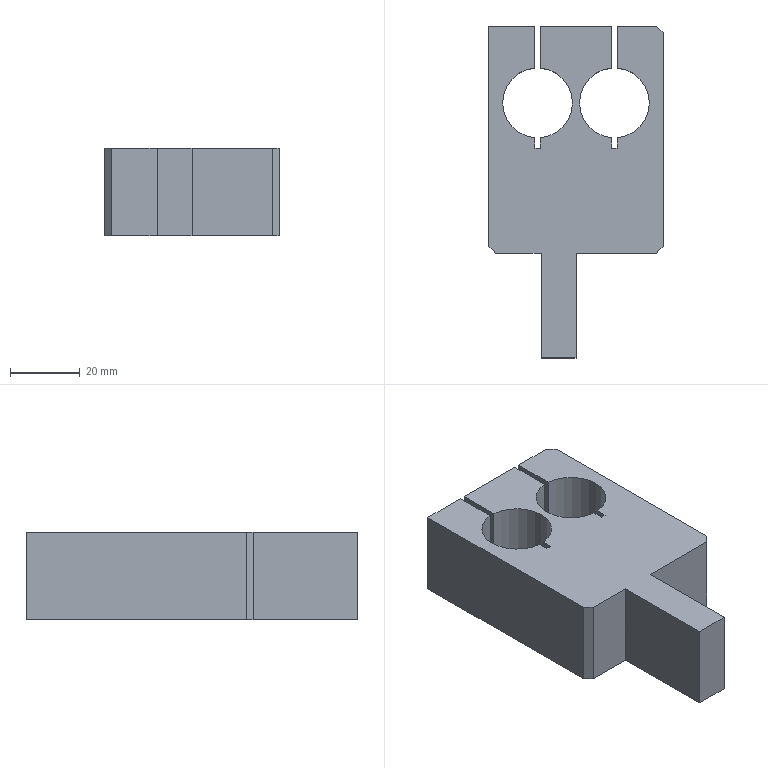Part | STEP file | 2012-06-08-010 | 1 solid | 31 faces | box 50 x 95 x 25 mm | volume 71766 mm3 | plane 25 | cylinder 6 | commonest cylinder face diameters 20 x6